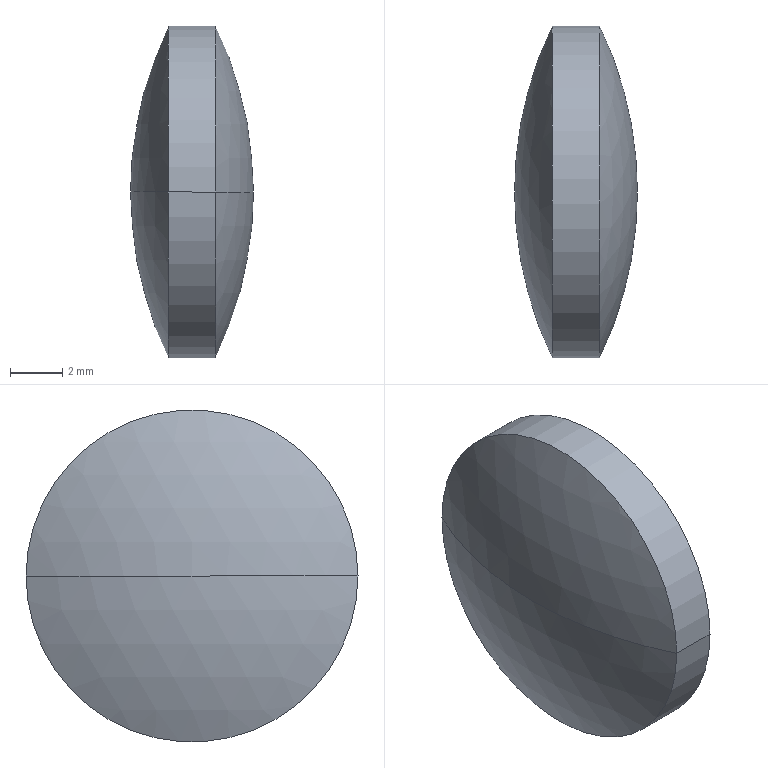Part | SolidWorks | features Revolution 1 | 1 solid | 6 faces | box 4.7 x 12.7 x 12.7 mm | volume 415.033 mm3 | sphere 4 | cylinder 2 | commonest cylinder face diameters 12.7 x2
STEP:
#1=CARTESIAN_POINT('',(11.389,6.35,0.));
#2=VERTEX_POINT('',#1);
#3=CARTESIAN_POINT('',(11.389,-6.35,0.));
#4=VERTEX_POINT('',#3);
#5=CARTESIAN_POINT('',(11.389,0.,0.));
#6=DIRECTION('',(1.,0.,0.));
#7=DIRECTION('',(0.,1.,0.));
#8=AXIS2_PLACEMENT_3D('',#5,#6,#7);
#9=CIRCLE('',#8,6.35);
#10=EDGE_CURVE('',#2,#4,#9,.T.);
#11=ORIENTED_EDGE('',*,*,#10,.T.);
#12=CARTESIAN_POINT('',(13.191,-6.35,0.));
#13=VERTEX_POINT('',#12);
#14=CARTESIAN_POINT('',(14.64,-6.35,0.));
#15=DIRECTION('',(1.,0.,0.));
#16=VECTOR('',#15,1000.);
#17=LINE('',#14,#16);
#18=EDGE_CURVE('',#4,#13,#17,.T.);
#19=ORIENTED_EDGE('',*,*,#18,.T.);
#20=CARTESIAN_POINT('',(13.191,6.35,0.));
#21=VERTEX_POINT('',#20);
#22=CARTESIAN_POINT('',(13.191,0.,0.));
#23=DIRECTION('',(1.,0.,0.));
#24=DIRECTION('',(0.,1.,0.));
#25=AXIS2_PLACEMENT_3D('',#22,#23,#24);
#26=CIRCLE('',#25,6.35);
#27=EDGE_CURVE('',#21,#13,#26,.T.);
#28=ORIENTED_EDGE('',*,*,#27,.F.);
#29=CARTESIAN_POINT('',(14.64,6.35,0.));
#30=DIRECTION('',(1.,0.,0.));
#31=VECTOR('',#30,1000.);
#32=LINE('',#29,#31);
#33=EDGE_CURVE('',#2,#21,#32,.T.);
#34=ORIENTED_EDGE('',*,*,#33,.F.);
#35=EDGE_LOOP('',(#11,#19,#28,#34));
#36=FACE_OUTER_BOUND('',#35,.T.);
#37=CARTESIAN_POINT('',(14.64,0.,0.));
#38=DIRECTION('',(1.,0.,0.));
#39=DIRECTION('',(0.,1.,0.));
#40=AXIS2_PLACEMENT_3D('',#37,#38,#39);
#41=CYLINDRICAL_SURFACE('',#40,6.35);
#42=ADVANCED_FACE('',(#36),#41,.T.);
#43=CARTESIAN_POINT('',(13.191,0.,0.));
#44=DIRECTION('',(1.,0.,0.));
#45=DIRECTION('',(0.,1.,0.));
#46=AXIS2_PLACEMENT_3D('',#43,#44,#45);
#47=CIRCLE('',#46,6.35);
#48=EDGE_CURVE('',#13,#21,#47,.T.);
#49=ORIENTED_EDGE('',*,*,#48,.T.);
#50=CARTESIAN_POINT('',(14.64,0.,0.));
#51=VERTEX_POINT('',#50);
#52=CARTESIAN_POINT('',(0.,0.,0.));
#53=DIRECTION('',(0.,0.,-1.));
#54=DIRECTION('',(0.,1.,0.));
#55=AXIS2_PLACEMENT_3D('',#52,#53,#54);
#56=CIRCLE('',#55,14.64);
#57=EDGE_CURVE('',#21,#51,#56,.T.);
#58=ORIENTED_EDGE('',*,*,#57,.T.);
#59=CARTESIAN_POINT('',(0.,0.,0.));
#60=DIRECTION('',(0.,0.,1.));
#61=DIRECTION('',(1.,0.,0.));
#62=AXIS2_PLACEMENT_3D('',#59,#60,#61);
#63=CIRCLE('',#62,14.64);
#64=EDGE_CURVE('',#13,#51,#63,.T.);
#65=ORIENTED_EDGE('',*,*,#64,.F.);
#66=EDGE_LOOP('',(#49,#58,#65));
#67=FACE_OUTER_BOUND('',#66,.T.);
#68=CARTESIAN_POINT('',(0.,0.,0.));
#69=DIRECTION('',(0.,0.,-1.));
#70=DIRECTION('',(0.,-1.,0.));
#71=AXIS2_PLACEMENT_3D('',#68,#69,#70);
#72=SPHERICAL_SURFACE('',#71,14.64);
#73=ADVANCED_FACE('',(#67),#72,.T.);
#74=CARTESIAN_POINT('',(9.94,0.,0.));
#75=VERTEX_POINT('',#74);
#76=CARTESIAN_POINT('',(24.58,0.,0.));
#77=DIRECTION('',(0.,0.,-1.));
#78=DIRECTION('',(-1.,0.,0.));
#79=AXIS2_PLACEMENT_3D('',#76,#77,#78);
#80=CIRCLE('',#79,14.64);
#81=EDGE_CURVE('',#75,#2,#80,.T.);
#82=ORIENTED_EDGE('',*,*,#81,.F.);
#83=CARTESIAN_POINT('',(24.58,0.,0.));
#84=DIRECTION('',(0.,0.,1.));
#85=DIRECTION('',(0.,-1.,0.));
#86=AXIS2_PLACEMENT_3D('',#83,#84,#85);
#87=CIRCLE('',#86,14.64);
#88=EDGE_CURVE('',#75,#4,#87,.T.);
#89=ORIENTED_EDGE('',*,*,#88,.T.);
#90=ORIENTED_EDGE('',*,*,#10,.F.);
#91=EDGE_LOOP('',(#82,#89,#90));
#92=FACE_OUTER_BOUND('',#91,.T.);
#93=CARTESIAN_POINT('',(24.58,0.,0.));
#94=DIRECTION('',(0.,0.,1.));
#95=DIRECTION('',(0.,1.,0.));
#96=AXIS2_PLACEMENT_3D('',#93,#94,#95);
#97=SPHERICAL_SURFACE('',#96,14.64);
#98=ADVANCED_FACE('',(#92),#97,.T.);
#99=ORIENTED_EDGE('',*,*,#88,.F.);
#100=ORIENTED_EDGE('',*,*,#81,.T.);
#101=CARTESIAN_POINT('',(11.389,0.,0.));
#102=DIRECTION('',(1.,0.,0.));
#103=DIRECTION('',(0.,1.,0.));
#104=AXIS2_PLACEMENT_3D('',#101,#102,#103);
#105=CIRCLE('',#104,6.35);
#106=EDGE_CURVE('',#4,#2,#105,.T.);
#107=ORIENTED_EDGE('',*,*,#106,.F.);
#108=EDGE_LOOP('',(#99,#100,#107));
#109=FACE_OUTER_BOUND('',#108,.T.);
#110=CARTESIAN_POINT('',(24.58,0.,0.));
#111=DIRECTION('',(0.,0.,1.));
#112=DIRECTION('',(0.,1.,0.));
#113=AXIS2_PLACEMENT_3D('',#110,#111,#112);
#114=SPHERICAL_SURFACE('',#113,14.64);
#115=ADVANCED_FACE('',(#109),#114,.T.);
#116=ORIENTED_EDGE('',*,*,#57,.F.);
#117=ORIENTED_EDGE('',*,*,#27,.T.);
#118=ORIENTED_EDGE('',*,*,#64,.T.);
#119=EDGE_LOOP('',(#116,#117,#118));
#120=FACE_OUTER_BOUND('',#119,.T.);
#121=CARTESIAN_POINT('',(0.,0.,0.));
#122=DIRECTION('',(0.,0.,-1.));
#123=DIRECTION('',(0.,-1.,0.));
#124=AXIS2_PLACEMENT_3D('',#121,#122,#123);
#125=SPHERICAL_SURFACE('',#124,14.64);
#126=ADVANCED_FACE('',(#120),#125,.T.);
#127=ORIENTED_EDGE('',*,*,#18,.F.);
#128=ORIENTED_EDGE('',*,*,#106,.T.);
#129=ORIENTED_EDGE('',*,*,#33,.T.);
#130=ORIENTED_EDGE('',*,*,#48,.F.);
#131=EDGE_LOOP('',(#127,#128,#129,#130));
#132=FACE_OUTER_BOUND('',#131,.T.);
#133=CARTESIAN_POINT('',(14.64,0.,0.));
#134=DIRECTION('',(1.,0.,0.));
#135=DIRECTION('',(0.,1.,0.));
#136=AXIS2_PLACEMENT_3D('',#133,#134,#135);
#137=CYLINDRICAL_SURFACE('',#136,6.35);
#138=ADVANCED_FACE('',(#132),#137,.T.);
#139=CLOSED_SHELL('',(#42,#73,#98,#115,#126,#138));
#140=MANIFOLD_SOLID_BREP('',#139);
#141=CARTESIAN_POINT('',(0.,0.,0.));
#142=DIRECTION('',(0.,0.,1.));
#143=DIRECTION('',(1.,0.,0.));
#144=AXIS2_PLACEMENT_3D('',#141,#142,#143);
#145=(LENGTH_UNIT()NAMED_UNIT(*)SI_UNIT(.MILLI.,.METRE.));
#146=UNCERTAINTY_MEASURE_WITH_UNIT(LENGTH_MEASURE(0.00001),#145,'','');
#147=(NAMED_UNIT(*)PLANE_ANGLE_UNIT()SI_UNIT($,.RADIAN.));
#148=(NAMED_UNIT(*)SI_UNIT($,.STERADIAN.)SOLID_ANGLE_UNIT());
#149=(GEOMETRIC_REPRESENTATION_CONTEXT(3)GLOBAL_UNCERTAINTY_ASSIGNED_CONTEXT((#146))GLOBAL_UNIT_ASSIGNED_CONTEXT((#145,#147,#148))REPRESENTATION_CONTEXT('',''));
#150=ADVANCED_BREP_SHAPE_REPRESENTATION('',(#140,#144),#149);